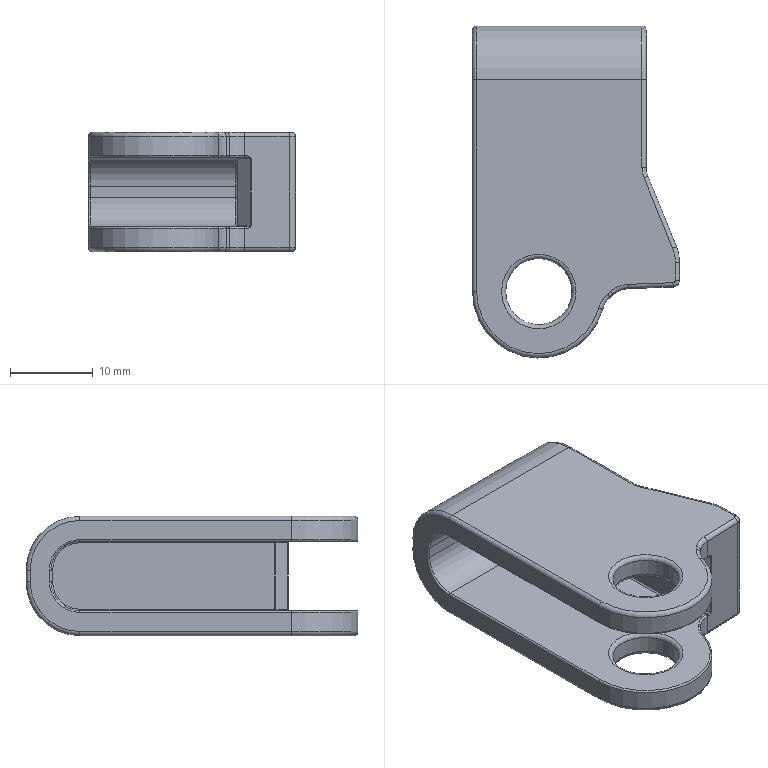Part | NX | features solid 2 | 1 solid | 92 faces | box 25 x 40.085 x 14.402 mm | volume 5792 mm3 | cylinder 43 | torus 32 | plane 15 | spline 2 | commonest cylinder face diameters 0.4 x14 1 x14 6 x5 7 x2 8 x2 13 x2